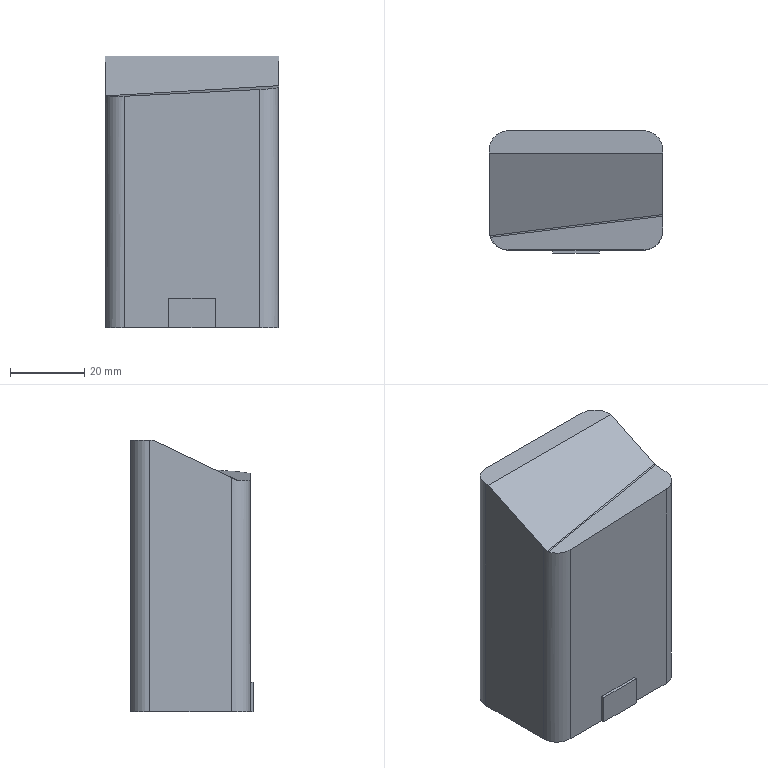Part | STEP file | gslz 2016.10.28-13_id1370_x_t | 1 solid | 17 faces | box 46.5 x 32.8 x 73 mm | volume 100113 mm3 | plane 11 | cylinder 4 | spline 2 | commonest cylinder face diameters 10 x4